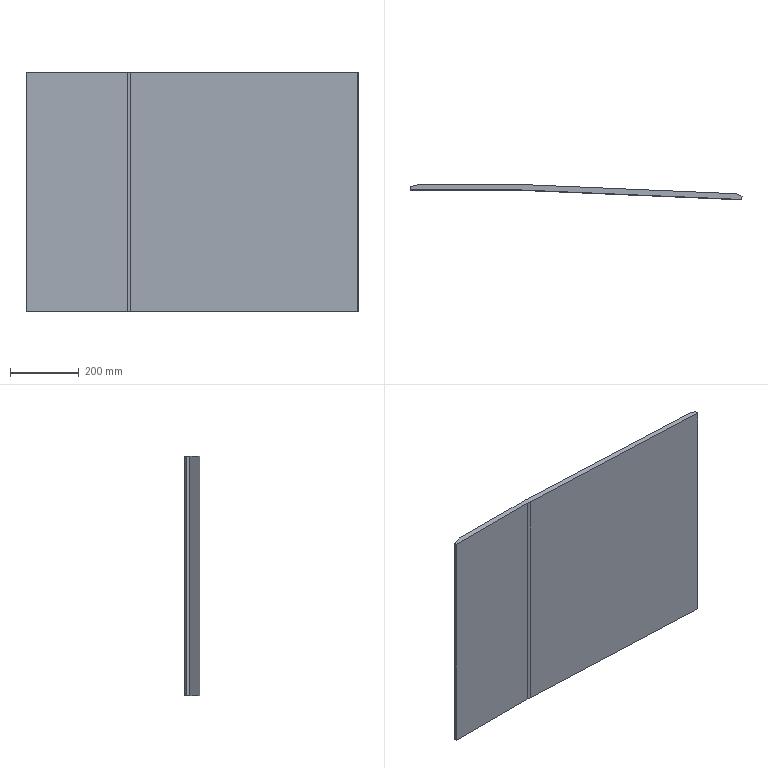Part | SolidWorks | features Extrusion 1, ICE 1 | 1 solid | 12 faces | box 968.586 x 44.7 x 700 mm | volume 10744321 mm3 | plane 10 | cylinder 2 | commonest cylinder face diameters 400 x1 432 x1
STEP:
#1=CARTESIAN_POINT('',(304.976,15.801,0.));
#2=VERTEX_POINT('',#1);
#3=CARTESIAN_POINT('',(295.707,16.,0.));
#4=VERTEX_POINT('',#3);
#5=CARTESIAN_POINT('',(295.707,-200.,0.));
#6=DIRECTION('',(0.,0.,1.));
#7=DIRECTION('',(1.,0.,0.));
#8=AXIS2_PLACEMENT_3D('',#5,#6,#7);
#9=CIRCLE('',#8,216.);
#10=EDGE_CURVE('',#2,#4,#9,.T.);
#11=ORIENTED_EDGE('',*,*,#10,.T.);
#12=CARTESIAN_POINT('',(295.707,16.,700.));
#13=VERTEX_POINT('',#12);
#14=CARTESIAN_POINT('',(295.707,16.,700.));
#15=DIRECTION('',(0.,0.,-1.));
#16=VECTOR('',#15,1000.);
#17=LINE('',#14,#16);
#18=EDGE_CURVE('',#13,#4,#17,.T.);
#19=ORIENTED_EDGE('',*,*,#18,.F.);
#20=CARTESIAN_POINT('',(304.976,15.801,700.));
#21=VERTEX_POINT('',#20);
#22=CARTESIAN_POINT('',(295.707,-200.,700.));
#23=DIRECTION('',(0.,0.,1.));
#24=DIRECTION('',(1.,0.,0.));
#25=AXIS2_PLACEMENT_3D('',#22,#23,#24);
#26=CIRCLE('',#25,216.);
#27=EDGE_CURVE('',#21,#13,#26,.T.);
#28=ORIENTED_EDGE('',*,*,#27,.F.);
#29=CARTESIAN_POINT('',(304.976,15.801,700.));
#30=DIRECTION('',(0.,0.,-1.));
#31=VECTOR('',#30,1000.);
#32=LINE('',#29,#31);
#33=EDGE_CURVE('',#21,#2,#32,.T.);
#34=ORIENTED_EDGE('',*,*,#33,.T.);
#35=EDGE_LOOP('',(#11,#19,#28,#34));
#36=FACE_OUTER_BOUND('',#35,.T.);
#37=CARTESIAN_POINT('',(295.707,-200.,700.));
#38=DIRECTION('',(0.,0.,-1.));
#39=DIRECTION('',(-1.,0.,0.));
#40=AXIS2_PLACEMENT_3D('',#37,#38,#39);
#41=CYLINDRICAL_SURFACE('',#40,216.);
#42=ADVANCED_FACE('',(#36),#41,.T.);
#43=CARTESIAN_POINT('',(30.,16.,0.));
#44=VERTEX_POINT('',#43);
#45=CARTESIAN_POINT('',(30.,16.,0.));
#46=DIRECTION('',(-1.,0.,0.));
#47=VECTOR('',#46,1000.);
#48=LINE('',#45,#47);
#49=EDGE_CURVE('',#4,#44,#48,.T.);
#50=ORIENTED_EDGE('',*,*,#49,.T.);
#51=CARTESIAN_POINT('',(30.,16.,700.));
#52=VERTEX_POINT('',#51);
#53=CARTESIAN_POINT('',(30.,16.,700.));
#54=DIRECTION('',(0.,0.,-1.));
#55=VECTOR('',#54,1000.);
#56=LINE('',#53,#55);
#57=EDGE_CURVE('',#52,#44,#56,.T.);
#58=ORIENTED_EDGE('',*,*,#57,.F.);
#59=CARTESIAN_POINT('',(30.,16.,700.));
#60=DIRECTION('',(-1.,0.,0.));
#61=VECTOR('',#60,1000.);
#62=LINE('',#59,#61);
#63=EDGE_CURVE('',#13,#52,#62,.T.);
#64=ORIENTED_EDGE('',*,*,#63,.F.);
#65=ORIENTED_EDGE('',*,*,#18,.T.);
#66=EDGE_LOOP('',(#50,#58,#64,#65));
#67=FACE_OUTER_BOUND('',#66,.T.);
#68=CARTESIAN_POINT('',(30.,16.,700.));
#69=DIRECTION('',(0.,-1.,0.));
#70=DIRECTION('',(0.,0.,-1.));
#71=AXIS2_PLACEMENT_3D('',#68,#69,#70);
#72=PLANE('',#71);
#73=ADVANCED_FACE('',(#67),#72,.F.);
#74=CARTESIAN_POINT('',(0.,9.,0.));
#75=VERTEX_POINT('',#74);
#76=CARTESIAN_POINT('',(0.,9.,0.));
#77=DIRECTION('',(-0.9738,-0.2272,0.));
#78=VECTOR('',#77,1000.);
#79=LINE('',#76,#78);
#80=EDGE_CURVE('',#44,#75,#79,.T.);
#81=ORIENTED_EDGE('',*,*,#80,.T.);
#82=CARTESIAN_POINT('',(0.,9.,700.));
#83=VERTEX_POINT('',#82);
#84=CARTESIAN_POINT('',(0.,9.,700.));
#85=DIRECTION('',(0.,0.,-1.));
#86=VECTOR('',#85,1000.);
#87=LINE('',#84,#86);
#88=EDGE_CURVE('',#83,#75,#87,.T.);
#89=ORIENTED_EDGE('',*,*,#88,.F.);
#90=CARTESIAN_POINT('',(0.,9.,700.));
#91=DIRECTION('',(-0.9738,-0.2272,0.));
#92=VECTOR('',#91,1000.);
#93=LINE('',#90,#92);
#94=EDGE_CURVE('',#52,#83,#93,.T.);
#95=ORIENTED_EDGE('',*,*,#94,.F.);
#96=ORIENTED_EDGE('',*,*,#57,.T.);
#97=EDGE_LOOP('',(#81,#89,#95,#96));
#98=FACE_OUTER_BOUND('',#97,.T.);
#99=CARTESIAN_POINT('',(0.,9.,700.));
#100=DIRECTION('',(0.2272,-0.9738,0.));
#101=DIRECTION('',(0.9738,0.2272,0.));
#102=AXIS2_PLACEMENT_3D('',#99,#100,#101);
#103=PLANE('',#102);
#104=ADVANCED_FACE('',(#98),#103,.F.);
#105=CARTESIAN_POINT('',(0.,0.,0.));
#106=VERTEX_POINT('',#105);
#107=CARTESIAN_POINT('',(0.,0.,0.));
#108=DIRECTION('',(0.,-1.,0.));
#109=VECTOR('',#108,1000.);
#110=LINE('',#107,#109);
#111=EDGE_CURVE('',#75,#106,#110,.T.);
#112=ORIENTED_EDGE('',*,*,#111,.T.);
#113=CARTESIAN_POINT('',(0.,0.,700.));
#114=VERTEX_POINT('',#113);
#115=CARTESIAN_POINT('',(0.,0.,700.));
#116=DIRECTION('',(0.,0.,-1.));
#117=VECTOR('',#116,1000.);
#118=LINE('',#115,#117);
#119=EDGE_CURVE('',#114,#106,#118,.T.);
#120=ORIENTED_EDGE('',*,*,#119,.F.);
#121=CARTESIAN_POINT('',(0.,0.,700.));
#122=DIRECTION('',(0.,-1.,0.));
#123=VECTOR('',#122,1000.);
#124=LINE('',#121,#123);
#125=EDGE_CURVE('',#83,#114,#124,.T.);
#126=ORIENTED_EDGE('',*,*,#125,.F.);
#127=ORIENTED_EDGE('',*,*,#88,.T.);
#128=EDGE_LOOP('',(#112,#120,#126,#127));
#129=FACE_OUTER_BOUND('',#128,.T.);
#130=CARTESIAN_POINT('',(0.,0.,700.));
#131=DIRECTION('',(1.,0.,0.));
#132=DIRECTION('',(0.,0.,-1.));
#133=AXIS2_PLACEMENT_3D('',#130,#131,#132);
#134=PLANE('',#133);
#135=ADVANCED_FACE('',(#129),#134,.F.);
#136=CARTESIAN_POINT('',(295.707,0.,0.));
#137=VERTEX_POINT('',#136);
#138=CARTESIAN_POINT('',(0.,0.,0.));
#139=DIRECTION('',(1.,0.,0.));
#140=VECTOR('',#139,1000.);
#141=LINE('',#138,#140);
#142=EDGE_CURVE('',#106,#137,#141,.T.);
#143=ORIENTED_EDGE('',*,*,#142,.T.);
#144=CARTESIAN_POINT('',(295.707,0.,700.));
#145=VERTEX_POINT('',#144);
#146=CARTESIAN_POINT('',(295.707,0.,700.));
#147=DIRECTION('',(0.,0.,-1.));
#148=VECTOR('',#147,1000.);
#149=LINE('',#146,#148);
#150=EDGE_CURVE('',#145,#137,#149,.T.);
#151=ORIENTED_EDGE('',*,*,#150,.F.);
#152=CARTESIAN_POINT('',(0.,0.,700.));
#153=DIRECTION('',(1.,0.,0.));
#154=VECTOR('',#153,1000.);
#155=LINE('',#152,#154);
#156=EDGE_CURVE('',#114,#145,#155,.T.);
#157=ORIENTED_EDGE('',*,*,#156,.F.);
#158=ORIENTED_EDGE('',*,*,#119,.T.);
#159=EDGE_LOOP('',(#143,#151,#157,#158));
#160=FACE_OUTER_BOUND('',#159,.T.);
#161=CARTESIAN_POINT('',(0.,0.,700.));
#162=DIRECTION('',(0.,1.,0.));
#163=DIRECTION('',(0.,0.,1.));
#164=AXIS2_PLACEMENT_3D('',#161,#162,#163);
#165=PLANE('',#164);
#166=ADVANCED_FACE('',(#160),#165,.F.);
#167=CARTESIAN_POINT('',(304.289,-0.1842,0.));
#168=VERTEX_POINT('',#167);
#169=CARTESIAN_POINT('',(295.707,-200.,0.));
#170=DIRECTION('',(0.,0.,-1.));
#171=DIRECTION('',(1.,0.,0.));
#172=AXIS2_PLACEMENT_3D('',#169,#170,#171);
#173=CIRCLE('',#172,200.);
#174=EDGE_CURVE('',#137,#168,#173,.T.);
#175=ORIENTED_EDGE('',*,*,#174,.T.);
#176=CARTESIAN_POINT('',(304.289,-0.1842,700.));
#177=VERTEX_POINT('',#176);
#178=CARTESIAN_POINT('',(304.289,-0.1842,700.));
#179=DIRECTION('',(0.,0.,-1.));
#180=VECTOR('',#179,1000.);
#181=LINE('',#178,#180);
#182=EDGE_CURVE('',#177,#168,#181,.T.);
#183=ORIENTED_EDGE('',*,*,#182,.F.);
#184=CARTESIAN_POINT('',(295.707,-200.,700.));
#185=DIRECTION('',(0.,0.,-1.));
#186=DIRECTION('',(1.,0.,0.));
#187=AXIS2_PLACEMENT_3D('',#184,#185,#186);
#188=CIRCLE('',#187,200.);
#189=EDGE_CURVE('',#145,#177,#188,.T.);
#190=ORIENTED_EDGE('',*,*,#189,.F.);
#191=ORIENTED_EDGE('',*,*,#150,.T.);
#192=EDGE_LOOP('',(#175,#183,#190,#191));
#193=FACE_OUTER_BOUND('',#192,.T.);
#194=CARTESIAN_POINT('',(295.707,-200.,700.));
#195=DIRECTION('',(0.,0.,-1.));
#196=DIRECTION('',(-1.,0.,0.));
#197=AXIS2_PLACEMENT_3D('',#194,#195,#196);
#198=CYLINDRICAL_SURFACE('',#197,200.);
#199=ADVANCED_FACE('',(#193),#198,.F.);
#200=CARTESIAN_POINT('',(968.2,-28.7,0.));
#201=VERTEX_POINT('',#200);
#202=CARTESIAN_POINT('',(304.289,-0.1842,0.));
#203=DIRECTION('',(0.9991,-0.04291,0.));
#204=VECTOR('',#203,1000.);
#205=LINE('',#202,#204);
#206=EDGE_CURVE('',#168,#201,#205,.T.);
#207=ORIENTED_EDGE('',*,*,#206,.T.);
#208=CARTESIAN_POINT('',(968.2,-28.7,700.));
#209=VERTEX_POINT('',#208);
#210=CARTESIAN_POINT('',(968.2,-28.7,700.));
#211=DIRECTION('',(0.,0.,-1.));
#212=VECTOR('',#211,1000.);
#213=LINE('',#210,#212);
#214=EDGE_CURVE('',#209,#201,#213,.T.);
#215=ORIENTED_EDGE('',*,*,#214,.F.);
#216=CARTESIAN_POINT('',(304.289,-0.1842,700.));
#217=DIRECTION('',(0.9991,-0.04291,0.));
#218=VECTOR('',#217,1000.);
#219=LINE('',#216,#218);
#220=EDGE_CURVE('',#177,#209,#219,.T.);
#221=ORIENTED_EDGE('',*,*,#220,.F.);
#222=ORIENTED_EDGE('',*,*,#182,.T.);
#223=EDGE_LOOP('',(#207,#215,#221,#222));
#224=FACE_OUTER_BOUND('',#223,.T.);
#225=CARTESIAN_POINT('',(304.289,-0.1842,700.));
#226=DIRECTION('',(0.04291,0.9991,0.));
#227=DIRECTION('',(-0.9991,0.04291,0.));
#228=AXIS2_PLACEMENT_3D('',#225,#226,#227);
#229=PLANE('',#228);
#230=ADVANCED_FACE('',(#224),#229,.F.);
#231=CARTESIAN_POINT('',(968.586,-19.708,0.));
#232=VERTEX_POINT('',#231);
#233=CARTESIAN_POINT('',(968.2,-28.7,0.));
#234=DIRECTION('',(0.04291,0.9991,0.));
#235=VECTOR('',#234,1000.);
#236=LINE('',#233,#235);
#237=EDGE_CURVE('',#201,#232,#236,.T.);
#238=ORIENTED_EDGE('',*,*,#237,.T.);
#239=CARTESIAN_POINT('',(968.586,-19.708,700.));
#240=VERTEX_POINT('',#239);
#241=CARTESIAN_POINT('',(968.586,-19.708,700.));
#242=DIRECTION('',(0.,0.,-1.));
#243=VECTOR('',#242,1000.);
#244=LINE('',#241,#243);
#245=EDGE_CURVE('',#240,#232,#244,.T.);
#246=ORIENTED_EDGE('',*,*,#245,.F.);
#247=CARTESIAN_POINT('',(968.2,-28.7,700.));
#248=DIRECTION('',(0.04291,0.9991,0.));
#249=VECTOR('',#248,1000.);
#250=LINE('',#247,#249);
#251=EDGE_CURVE('',#209,#240,#250,.T.);
#252=ORIENTED_EDGE('',*,*,#251,.F.);
#253=ORIENTED_EDGE('',*,*,#214,.T.);
#254=EDGE_LOOP('',(#238,#246,#252,#253));
#255=FACE_OUTER_BOUND('',#254,.T.);
#256=CARTESIAN_POINT('',(968.2,-28.7,700.));
#257=DIRECTION('',(-0.9991,0.04291,0.));
#258=DIRECTION('',(-0.04291,-0.9991,0.));
#259=AXIS2_PLACEMENT_3D('',#256,#257,#258);
#260=PLANE('',#259);
#261=ADVANCED_FACE('',(#255),#260,.F.);
#262=CARTESIAN_POINT('',(953.9,-12.071,0.));
#263=VERTEX_POINT('',#262);
#264=CARTESIAN_POINT('',(953.9,-12.071,0.));
#265=DIRECTION('',(-0.8872,0.4614,0.));
#266=VECTOR('',#265,1000.);
#267=LINE('',#264,#266);
#268=EDGE_CURVE('',#232,#263,#267,.T.);
#269=ORIENTED_EDGE('',*,*,#268,.T.);
#270=CARTESIAN_POINT('',(953.9,-12.071,700.));
#271=VERTEX_POINT('',#270);
#272=CARTESIAN_POINT('',(953.9,-12.071,700.));
#273=DIRECTION('',(0.,0.,-1.));
#274=VECTOR('',#273,1000.);
#275=LINE('',#272,#274);
#276=EDGE_CURVE('',#271,#263,#275,.T.);
#277=ORIENTED_EDGE('',*,*,#276,.F.);
#278=CARTESIAN_POINT('',(953.9,-12.071,700.));
#279=DIRECTION('',(-0.8872,0.4614,0.));
#280=VECTOR('',#279,1000.);
#281=LINE('',#278,#280);
#282=EDGE_CURVE('',#240,#271,#281,.T.);
#283=ORIENTED_EDGE('',*,*,#282,.F.);
#284=ORIENTED_EDGE('',*,*,#245,.T.);
#285=EDGE_LOOP('',(#269,#277,#283,#284));
#286=FACE_OUTER_BOUND('',#285,.T.);
#287=CARTESIAN_POINT('',(953.9,-12.071,700.));
#288=DIRECTION('',(-0.4614,-0.8872,0.));
#289=DIRECTION('',(0.8872,-0.4614,0.));
#290=AXIS2_PLACEMENT_3D('',#287,#288,#289);
#291=PLANE('',#290);
#292=ADVANCED_FACE('',(#286),#291,.F.);
#293=CARTESIAN_POINT('',(304.976,15.801,0.));
#294=DIRECTION('',(-0.9991,0.04291,0.));
#295=VECTOR('',#294,1000.);
#296=LINE('',#293,#295);
#297=EDGE_CURVE('',#263,#2,#296,.T.);
#298=ORIENTED_EDGE('',*,*,#297,.T.);
#299=ORIENTED_EDGE('',*,*,#33,.F.);
#300=CARTESIAN_POINT('',(304.976,15.801,700.));
#301=DIRECTION('',(-0.9991,0.04291,0.));
#302=VECTOR('',#301,1000.);
#303=LINE('',#300,#302);
#304=EDGE_CURVE('',#271,#21,#303,.T.);
#305=ORIENTED_EDGE('',*,*,#304,.F.);
#306=ORIENTED_EDGE('',*,*,#276,.T.);
#307=EDGE_LOOP('',(#298,#299,#305,#306));
#308=FACE_OUTER_BOUND('',#307,.T.);
#309=CARTESIAN_POINT('',(304.976,15.801,700.));
#310=DIRECTION('',(-0.04291,-0.9991,0.));
#311=DIRECTION('',(0.9991,-0.04291,0.));
#312=AXIS2_PLACEMENT_3D('',#309,#310,#311);
#313=PLANE('',#312);
#314=ADVANCED_FACE('',(#308),#313,.F.);
#315=ORIENTED_EDGE('',*,*,#27,.T.);
#316=ORIENTED_EDGE('',*,*,#63,.T.);
#317=ORIENTED_EDGE('',*,*,#94,.T.);
#318=ORIENTED_EDGE('',*,*,#125,.T.);
#319=ORIENTED_EDGE('',*,*,#156,.T.);
#320=ORIENTED_EDGE('',*,*,#189,.T.);
#321=ORIENTED_EDGE('',*,*,#220,.T.);
#322=ORIENTED_EDGE('',*,*,#251,.T.);
#323=ORIENTED_EDGE('',*,*,#282,.T.);
#324=ORIENTED_EDGE('',*,*,#304,.T.);
#325=EDGE_LOOP('',(#315,#316,#317,#318,#319,#320,#321,#322,#323,#324));
#326=FACE_OUTER_BOUND('',#325,.T.);
#327=CARTESIAN_POINT('',(295.707,-200.,700.));
#328=DIRECTION('',(0.,0.,1.));
#329=DIRECTION('',(1.,0.,0.));
#330=AXIS2_PLACEMENT_3D('',#327,#328,#329);
#331=PLANE('',#330);
#332=ADVANCED_FACE('',(#326),#331,.T.);
#333=ORIENTED_EDGE('',*,*,#10,.F.);
#334=ORIENTED_EDGE('',*,*,#297,.F.);
#335=ORIENTED_EDGE('',*,*,#268,.F.);
#336=ORIENTED_EDGE('',*,*,#237,.F.);
#337=ORIENTED_EDGE('',*,*,#206,.F.);
#338=ORIENTED_EDGE('',*,*,#174,.F.);
#339=ORIENTED_EDGE('',*,*,#142,.F.);
#340=ORIENTED_EDGE('',*,*,#111,.F.);
#341=ORIENTED_EDGE('',*,*,#80,.F.);
#342=ORIENTED_EDGE('',*,*,#49,.F.);
#343=EDGE_LOOP('',(#333,#334,#335,#336,#337,#338,#339,#340,#341,#342));
#344=FACE_OUTER_BOUND('',#343,.T.);
#345=CARTESIAN_POINT('',(295.707,-200.,0.));
#346=DIRECTION('',(0.,0.,1.));
#347=DIRECTION('',(1.,0.,0.));
#348=AXIS2_PLACEMENT_3D('',#345,#346,#347);
#349=PLANE('',#348);
#350=ADVANCED_FACE('',(#344),#349,.F.);
#351=CLOSED_SHELL('',(#42,#73,#104,#135,#166,#199,#230,#261,#292,#314,#332,#350));
#352=MANIFOLD_SOLID_BREP('',#351);
#353=CARTESIAN_POINT('',(0.,0.,0.));
#354=DIRECTION('',(0.,0.,1.));
#355=DIRECTION('',(1.,0.,0.));
#356=AXIS2_PLACEMENT_3D('',#353,#354,#355);
#357=(LENGTH_UNIT()NAMED_UNIT(*)SI_UNIT(.MILLI.,.METRE.));
#358=UNCERTAINTY_MEASURE_WITH_UNIT(LENGTH_MEASURE(0.00001),#357,'','');
#359=(NAMED_UNIT(*)PLANE_ANGLE_UNIT()SI_UNIT($,.RADIAN.));
#360=(NAMED_UNIT(*)SI_UNIT($,.STERADIAN.)SOLID_ANGLE_UNIT());
#361=(GEOMETRIC_REPRESENTATION_CONTEXT(3)GLOBAL_UNCERTAINTY_ASSIGNED_CONTEXT((#358))GLOBAL_UNIT_ASSIGNED_CONTEXT((#357,#359,#360))REPRESENTATION_CONTEXT('',''));
#362=ADVANCED_BREP_SHAPE_REPRESENTATION('',(#352,#356),#361);